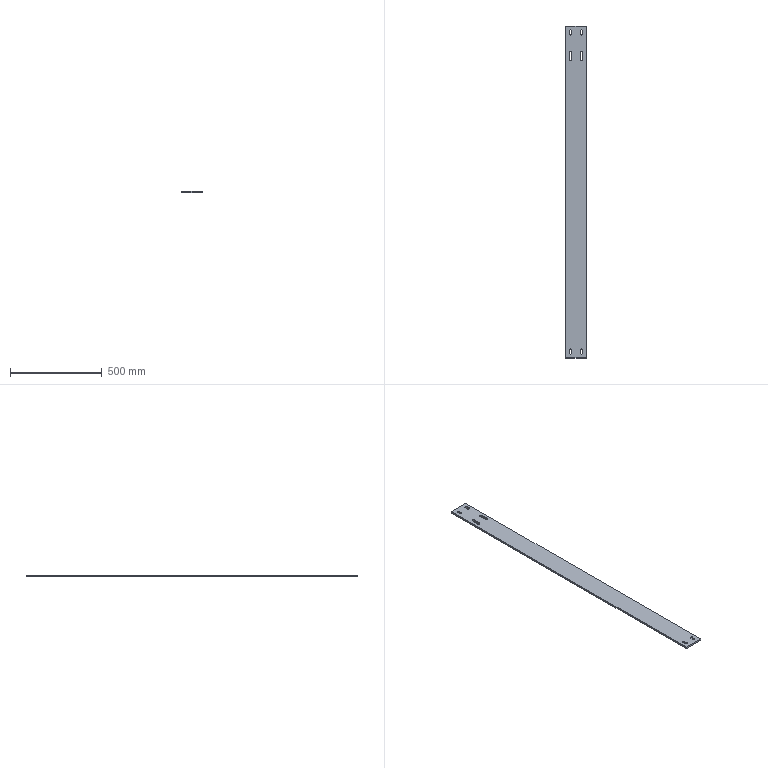Part | STEP file | Connecting plate | 1 solid | 30 faces | box 110 x 1805 x 10 mm | volume 1957224 mm3 | plane 18 | cylinder 12 | commonest cylinder face diameters 14 x12